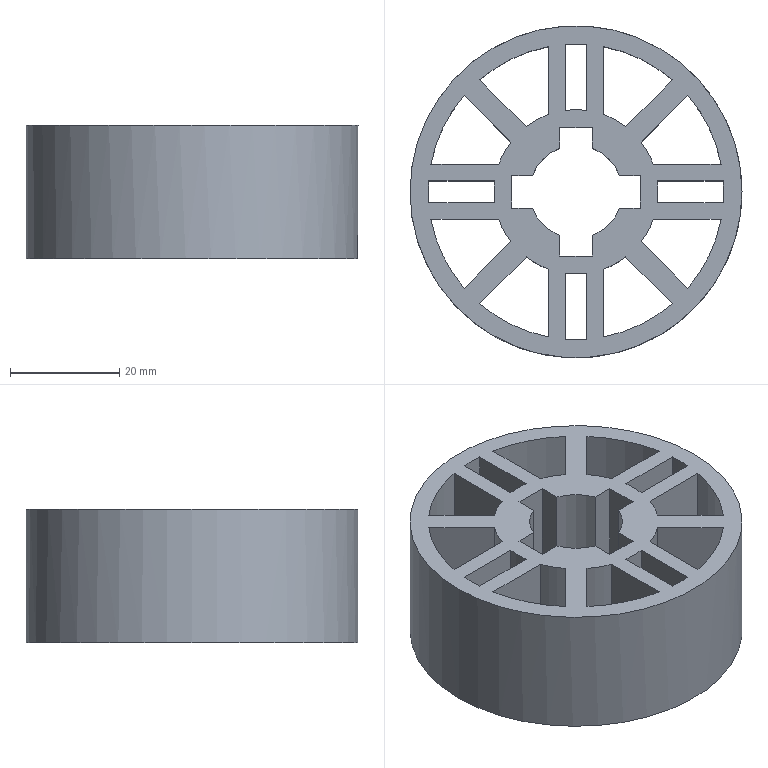Part | NX | features DATUM_CSYS 1, EXTRUDE 1, LINKED_FACE 1, SKETCH 1 | 1 solid | 67 faces | box 60.7 x 60.7 x 24.4 mm | volume 36264 mm3 | plane 38 | cylinder 29 | commonest cylinder face diameters 30 x12 54 x12 17 x4 60.7 x1